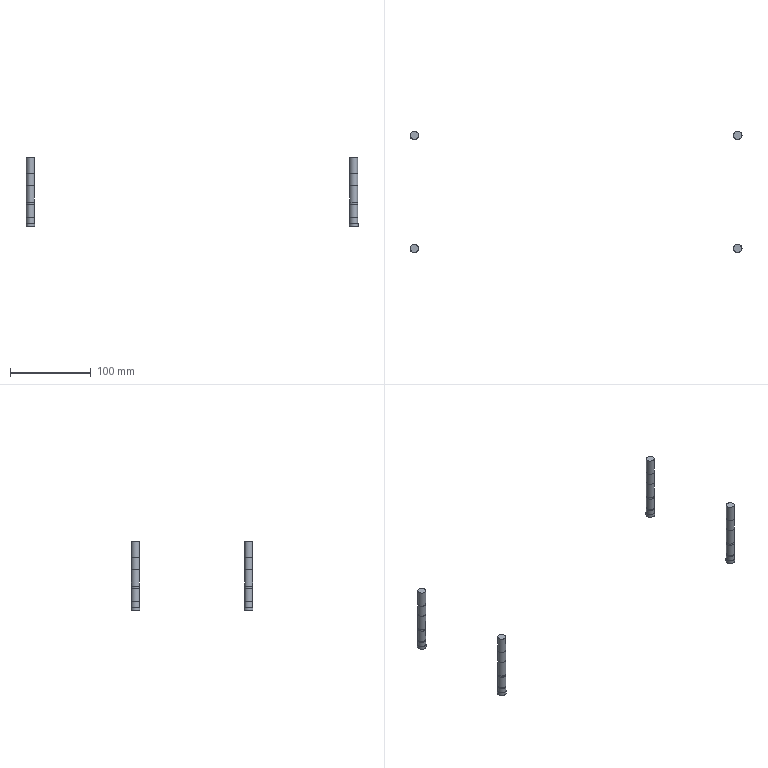Part | NX | features BREP 2 | 8 solids | 56 faces | box 410.8 x 150.8 x 85 mm | volume 33105 mm3 | plane 28 | cylinder 20 | torus 4 | cone 4 | commonest cylinder face diameters 10 x8 10.008 x4 10.1 x4 10.8 x4